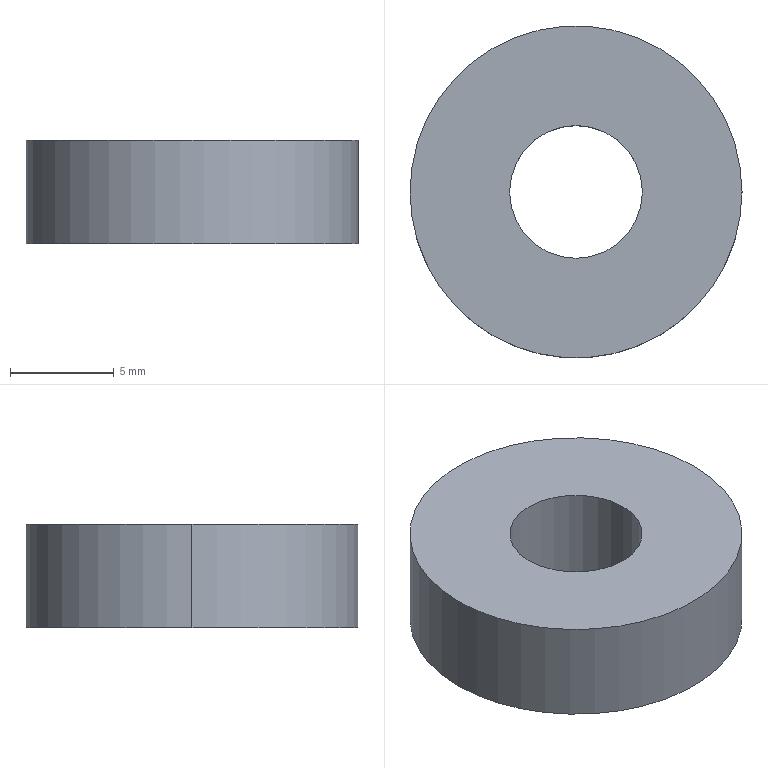Part | SolidWorks | features Extrusion 1 | 1 solid | 6 faces | box 16 x 16 x 5 mm | volume 844.46 mm3 | cylinder 4 | plane 2 | commonest cylinder face diameters 6.4 x2 16 x2
STEP:
#1=CARTESIAN_POINT('',(-3.2,0.,-2.5));
#2=VERTEX_POINT('',#1);
#3=CARTESIAN_POINT('',(3.2,0.,-2.5));
#4=VERTEX_POINT('',#3);
#5=CARTESIAN_POINT('',(0.,0.,-2.5));
#6=DIRECTION('',(0.,0.,1.));
#7=DIRECTION('',(1.,0.,0.));
#8=AXIS2_PLACEMENT_3D('',#5,#6,#7);
#9=CIRCLE('',#8,3.2);
#10=EDGE_CURVE('',#2,#4,#9,.T.);
#11=ORIENTED_EDGE('',*,*,#10,.F.);
#12=CARTESIAN_POINT('',(-3.2,0.,2.5));
#13=VERTEX_POINT('',#12);
#14=CARTESIAN_POINT('',(-3.2,0.,-2.5));
#15=DIRECTION('',(0.,0.,1.));
#16=VECTOR('',#15,1000.);
#17=LINE('',#14,#16);
#18=EDGE_CURVE('',#2,#13,#17,.T.);
#19=ORIENTED_EDGE('',*,*,#18,.T.);
#20=CARTESIAN_POINT('',(3.2,0.,2.5));
#21=VERTEX_POINT('',#20);
#22=CARTESIAN_POINT('',(0.,0.,2.5));
#23=DIRECTION('',(0.,0.,1.));
#24=DIRECTION('',(1.,0.,0.));
#25=AXIS2_PLACEMENT_3D('',#22,#23,#24);
#26=CIRCLE('',#25,3.2);
#27=EDGE_CURVE('',#13,#21,#26,.T.);
#28=ORIENTED_EDGE('',*,*,#27,.T.);
#29=CARTESIAN_POINT('',(3.2,0.,-2.5));
#30=DIRECTION('',(0.,0.,1.));
#31=VECTOR('',#30,1000.);
#32=LINE('',#29,#31);
#33=EDGE_CURVE('',#4,#21,#32,.T.);
#34=ORIENTED_EDGE('',*,*,#33,.F.);
#35=EDGE_LOOP('',(#11,#19,#28,#34));
#36=FACE_OUTER_BOUND('',#35,.T.);
#37=CARTESIAN_POINT('',(0.,0.,-2.5));
#38=DIRECTION('',(0.,0.,1.));
#39=DIRECTION('',(1.,0.,0.));
#40=AXIS2_PLACEMENT_3D('',#37,#38,#39);
#41=CYLINDRICAL_SURFACE('',#40,3.2);
#42=ADVANCED_FACE('',(#36),#41,.F.);
#43=CARTESIAN_POINT('',(8.,0.,-2.5));
#44=VERTEX_POINT('',#43);
#45=CARTESIAN_POINT('',(-8.,0.,-2.5));
#46=VERTEX_POINT('',#45);
#47=CARTESIAN_POINT('',(0.,0.,-2.5));
#48=DIRECTION('',(0.,0.,1.));
#49=DIRECTION('',(1.,0.,0.));
#50=AXIS2_PLACEMENT_3D('',#47,#48,#49);
#51=CIRCLE('',#50,8.);
#52=EDGE_CURVE('',#44,#46,#51,.T.);
#53=ORIENTED_EDGE('',*,*,#52,.T.);
#54=CARTESIAN_POINT('',(-8.,0.,2.5));
#55=VERTEX_POINT('',#54);
#56=CARTESIAN_POINT('',(-8.,0.,-2.5));
#57=DIRECTION('',(0.,0.,1.));
#58=VECTOR('',#57,1000.);
#59=LINE('',#56,#58);
#60=EDGE_CURVE('',#46,#55,#59,.T.);
#61=ORIENTED_EDGE('',*,*,#60,.T.);
#62=CARTESIAN_POINT('',(8.,0.,2.5));
#63=VERTEX_POINT('',#62);
#64=CARTESIAN_POINT('',(0.,0.,2.5));
#65=DIRECTION('',(0.,0.,1.));
#66=DIRECTION('',(1.,0.,0.));
#67=AXIS2_PLACEMENT_3D('',#64,#65,#66);
#68=CIRCLE('',#67,8.);
#69=EDGE_CURVE('',#63,#55,#68,.T.);
#70=ORIENTED_EDGE('',*,*,#69,.F.);
#71=CARTESIAN_POINT('',(8.,0.,-2.5));
#72=DIRECTION('',(0.,0.,1.));
#73=VECTOR('',#72,1000.);
#74=LINE('',#71,#73);
#75=EDGE_CURVE('',#44,#63,#74,.T.);
#76=ORIENTED_EDGE('',*,*,#75,.F.);
#77=EDGE_LOOP('',(#53,#61,#70,#76));
#78=FACE_OUTER_BOUND('',#77,.T.);
#79=CARTESIAN_POINT('',(0.,0.,-2.5));
#80=DIRECTION('',(0.,0.,1.));
#81=DIRECTION('',(1.,0.,0.));
#82=AXIS2_PLACEMENT_3D('',#79,#80,#81);
#83=CYLINDRICAL_SURFACE('',#82,8.);
#84=ADVANCED_FACE('',(#78),#83,.T.);
#85=ORIENTED_EDGE('',*,*,#60,.F.);
#86=CARTESIAN_POINT('',(0.,0.,-2.5));
#87=DIRECTION('',(0.,0.,1.));
#88=DIRECTION('',(1.,0.,0.));
#89=AXIS2_PLACEMENT_3D('',#86,#87,#88);
#90=CIRCLE('',#89,8.);
#91=EDGE_CURVE('',#46,#44,#90,.T.);
#92=ORIENTED_EDGE('',*,*,#91,.T.);
#93=ORIENTED_EDGE('',*,*,#75,.T.);
#94=CARTESIAN_POINT('',(0.,0.,2.5));
#95=DIRECTION('',(0.,0.,1.));
#96=DIRECTION('',(1.,0.,0.));
#97=AXIS2_PLACEMENT_3D('',#94,#95,#96);
#98=CIRCLE('',#97,8.);
#99=EDGE_CURVE('',#55,#63,#98,.T.);
#100=ORIENTED_EDGE('',*,*,#99,.F.);
#101=EDGE_LOOP('',(#85,#92,#93,#100));
#102=FACE_OUTER_BOUND('',#101,.T.);
#103=CARTESIAN_POINT('',(0.,0.,-2.5));
#104=DIRECTION('',(0.,0.,1.));
#105=DIRECTION('',(1.,0.,0.));
#106=AXIS2_PLACEMENT_3D('',#103,#104,#105);
#107=CYLINDRICAL_SURFACE('',#106,8.);
#108=ADVANCED_FACE('',(#102),#107,.T.);
#109=CARTESIAN_POINT('',(0.,0.,-2.5));
#110=DIRECTION('',(0.,0.,1.));
#111=DIRECTION('',(1.,0.,0.));
#112=AXIS2_PLACEMENT_3D('',#109,#110,#111);
#113=CIRCLE('',#112,3.2);
#114=EDGE_CURVE('',#4,#2,#113,.T.);
#115=ORIENTED_EDGE('',*,*,#114,.T.);
#116=ORIENTED_EDGE('',*,*,#10,.T.);
#117=EDGE_LOOP('',(#115,#116));
#118=FACE_BOUND('',#117,.T.);
#119=ORIENTED_EDGE('',*,*,#52,.F.);
#120=ORIENTED_EDGE('',*,*,#91,.F.);
#121=EDGE_LOOP('',(#119,#120));
#122=FACE_OUTER_BOUND('',#121,.T.);
#123=CARTESIAN_POINT('',(0.,0.,-2.5));
#124=DIRECTION('',(0.,0.,1.));
#125=DIRECTION('',(1.,0.,0.));
#126=AXIS2_PLACEMENT_3D('',#123,#124,#125);
#127=PLANE('',#126);
#128=ADVANCED_FACE('',(#118,#122),#127,.F.);
#129=CARTESIAN_POINT('',(0.,0.,2.5));
#130=DIRECTION('',(0.,0.,1.));
#131=DIRECTION('',(1.,0.,0.));
#132=AXIS2_PLACEMENT_3D('',#129,#130,#131);
#133=CIRCLE('',#132,3.2);
#134=EDGE_CURVE('',#21,#13,#133,.T.);
#135=ORIENTED_EDGE('',*,*,#134,.F.);
#136=ORIENTED_EDGE('',*,*,#27,.F.);
#137=EDGE_LOOP('',(#135,#136));
#138=FACE_BOUND('',#137,.T.);
#139=ORIENTED_EDGE('',*,*,#69,.T.);
#140=ORIENTED_EDGE('',*,*,#99,.T.);
#141=EDGE_LOOP('',(#139,#140));
#142=FACE_OUTER_BOUND('',#141,.T.);
#143=CARTESIAN_POINT('',(0.,0.,2.5));
#144=DIRECTION('',(0.,0.,1.));
#145=DIRECTION('',(1.,0.,0.));
#146=AXIS2_PLACEMENT_3D('',#143,#144,#145);
#147=PLANE('',#146);
#148=ADVANCED_FACE('',(#138,#142),#147,.T.);
#149=ORIENTED_EDGE('',*,*,#18,.F.);
#150=ORIENTED_EDGE('',*,*,#114,.F.);
#151=ORIENTED_EDGE('',*,*,#33,.T.);
#152=ORIENTED_EDGE('',*,*,#134,.T.);
#153=EDGE_LOOP('',(#149,#150,#151,#152));
#154=FACE_OUTER_BOUND('',#153,.T.);
#155=CARTESIAN_POINT('',(0.,0.,-2.5));
#156=DIRECTION('',(0.,0.,1.));
#157=DIRECTION('',(1.,0.,0.));
#158=AXIS2_PLACEMENT_3D('',#155,#156,#157);
#159=CYLINDRICAL_SURFACE('',#158,3.2);
#160=ADVANCED_FACE('',(#154),#159,.F.);
#161=CLOSED_SHELL('',(#42,#84,#108,#128,#148,#160));
#162=MANIFOLD_SOLID_BREP('',#161);
#163=CARTESIAN_POINT('',(0.,0.,0.));
#164=DIRECTION('',(0.,0.,1.));
#165=DIRECTION('',(1.,0.,0.));
#166=AXIS2_PLACEMENT_3D('',#163,#164,#165);
#167=(LENGTH_UNIT()NAMED_UNIT(*)SI_UNIT(.MILLI.,.METRE.));
#168=UNCERTAINTY_MEASURE_WITH_UNIT(LENGTH_MEASURE(0.00001),#167,'','');
#169=(NAMED_UNIT(*)PLANE_ANGLE_UNIT()SI_UNIT($,.RADIAN.));
#170=(NAMED_UNIT(*)SI_UNIT($,.STERADIAN.)SOLID_ANGLE_UNIT());
#171=(GEOMETRIC_REPRESENTATION_CONTEXT(3)GLOBAL_UNCERTAINTY_ASSIGNED_CONTEXT((#168))GLOBAL_UNIT_ASSIGNED_CONTEXT((#167,#169,#170))REPRESENTATION_CONTEXT('',''));
#172=ADVANCED_BREP_SHAPE_REPRESENTATION('',(#162,#166),#171);